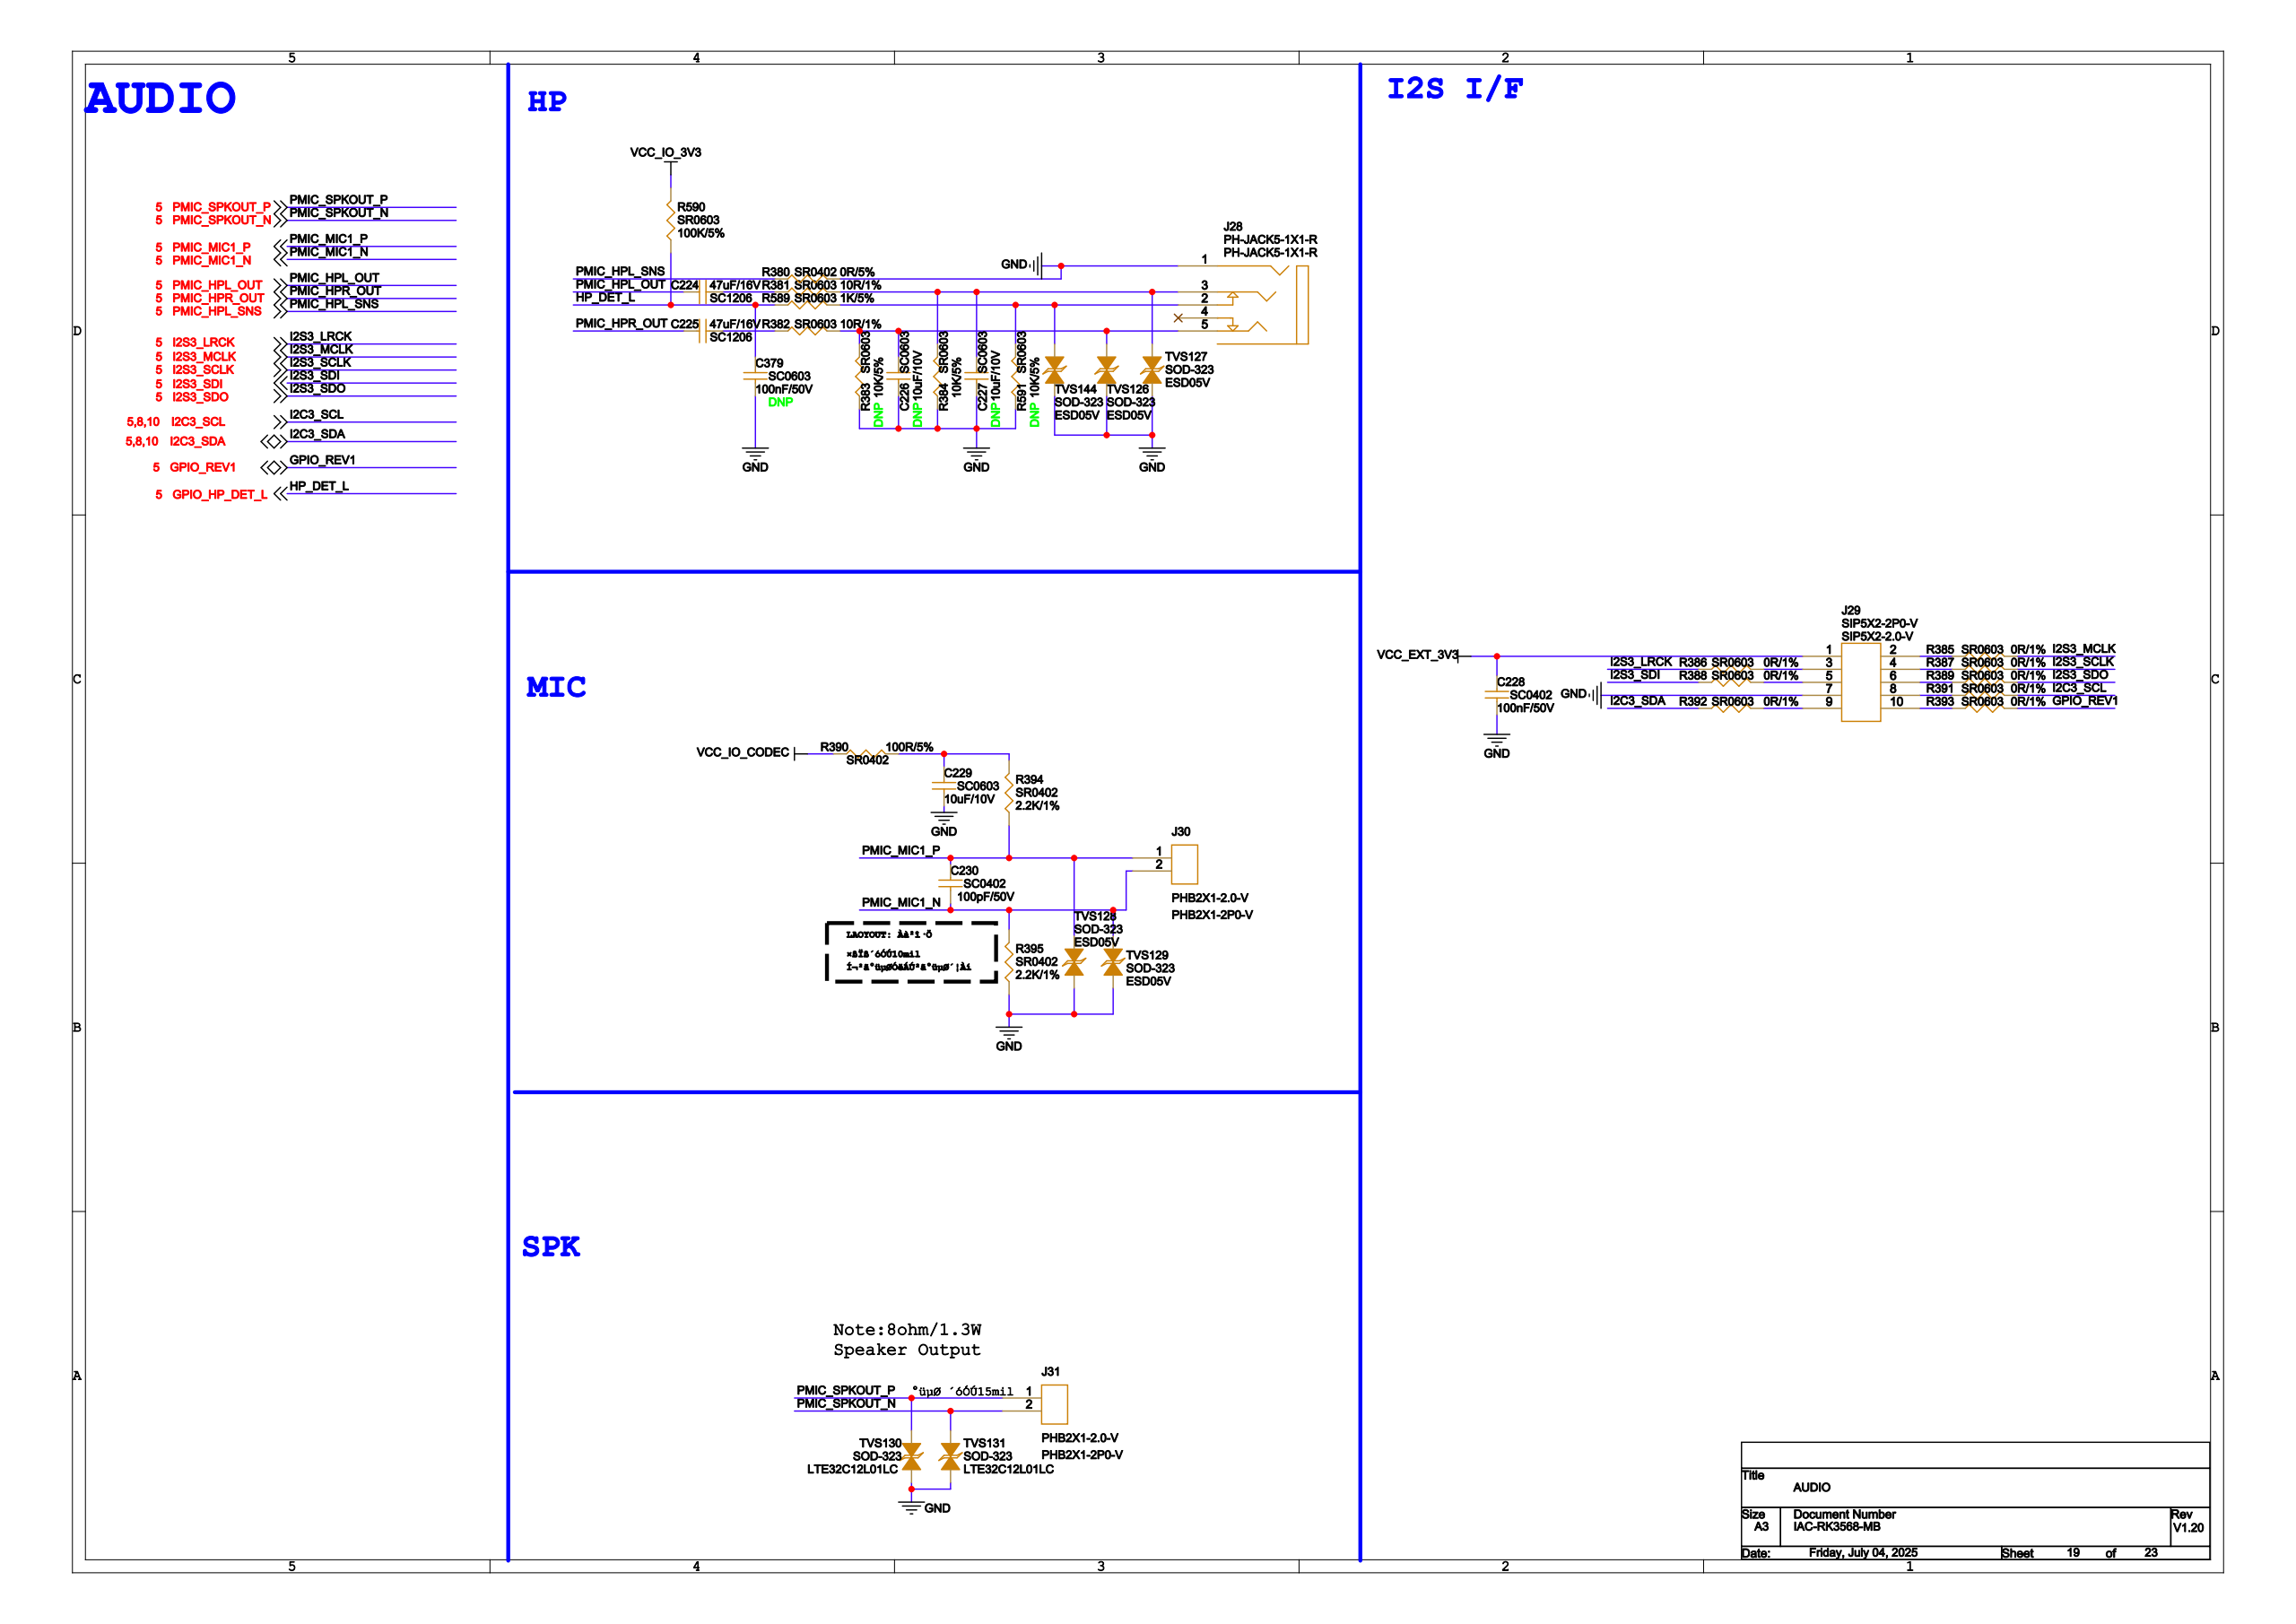Circuit board | Cadence Allegro | 1138 parts | 722 nets | one sheet of the schematic
Parts on this sheet (reference | value | footprint):
C224 | 47uF/16V | SC1206
C225 | 47uF/16V | SC1206
C226 | 10uF/10V | SC0603
C227 | 10uF/10V | SC0603
C228 | 100nF/50V | SC0402
C229 | 10uF/10V | SC0603
C230 | 100pF/50V | SC0402
C379 | 100nF/50V | SC0603
J28 | PH-JACK5-1X1-R | PH-JACK5-1X1-R
J29 | SIP5X2-2.0-V | SIP5X2-2P0-V
J30 | PHB2X1-2.0-V | PHB2X1-2P0-V
J31 | PHB2X1-2.0-V | PHB2X1-2P0-V
R380 | 0R/5% | SR0402
R381 | 10R/1% | SR0603
R382 | 10R/1% | SR0603
R383 | 10K/5% | SR0603
R384 | 10K/5% | SR0603
R385 | 0R/1% | SR0603
R386 | 0R/1% | SR0603
R387 | 0R/1% | SR0603
R388 | 0R/1% | SR0603
R389 | 0R/1% | SR0603
R390 | 100R/5% | SR0402
R391 | 0R/1% | SR0603
R392 | 0R/1% | SR0603
R393 | 0R/1% | SR0603
R394 | 2.2K/1% | SR0402
R395 | 2.2K/1% | SR0402
R589 | 1K/5% | SR0603
R590 | 100K/5% | SR0603
R591 | 10K/5% | SR0603
TVS126 | ESD05V | SOD-323
TVS127 | ESD05V | SOD-323
TVS128 | ESD05V | SOD-323
TVS129 | ESD05V | SOD-323
TVS130 | LTE32C12L01LC | SOD-323
TVS131 | LTE32C12L01LC | SOD-323
TVS144 | ESD05V | SOD-323
Nets of these parts (net: part-pin ...):
VCC_EXT_3V3: C228-1 J29-1
GND: C226-2 C227-2 C228-2 C229-2 C379-2 J28-1 J29-7 R380-2 R383-1 R384-1 R395-1 R591-1 TVS126-1 TVS127-1 TVS128-1 TVS129-1 TVS130-1 TVS131-1 TVS144-1
PMIC_HPL_OUT: C224-1
N203164: C224-2 R381-1
PMIC_HPR_OUT: C225-1
N203174: C225-2 R382-1
N202844: C226-1 J28-5 R382-2 R383-2 TVS126-2
N203104: C227-1 J28-3 R381-2 R384-2 TVS127-2
PMIC_MIC1_P: C230-1 J30-1 R394-1 TVS128-2
PMIC_MIC1_N: C230-2 J30-2 R395-2 TVS129-2
N5446948: J28-2 R589-2 R591-2 TVS144-2
VCC_IO_3V3: R590-2
N19622838: C229-1 R390-2 R394-2
GPIO_HP_DET_L: C379-1 R589-1 R590-1
N4708790: J29-10 R393-2
N4708616: J29-2 R385-2
N4708660: J29-3 R386-2
N4708664: J29-4 R387-2
N4708708: J29-5 R388-2
N4708712: J29-6 R389-2
N4708756: J29-8 R391-2
N4708760: J29-9 R392-2
PMIC_SPKOUT_P: J31-1 TVS130-2
PMIC_SPKOUT_N: J31-2 TVS131-2
VCC_IO_CODEC: R390-1
I2S3_SCLK: R387-1
I2S3_LRCK: R386-1
I2S3_SDO: R389-1
I2S3_SDI: R388-1
GPIO_REV1: R393-1
I2C3_SCL: R391-1
I2C3_SDA: R392-1
I2S3_MCLK: R385-1
PMIC_HPL_SNS: R380-1